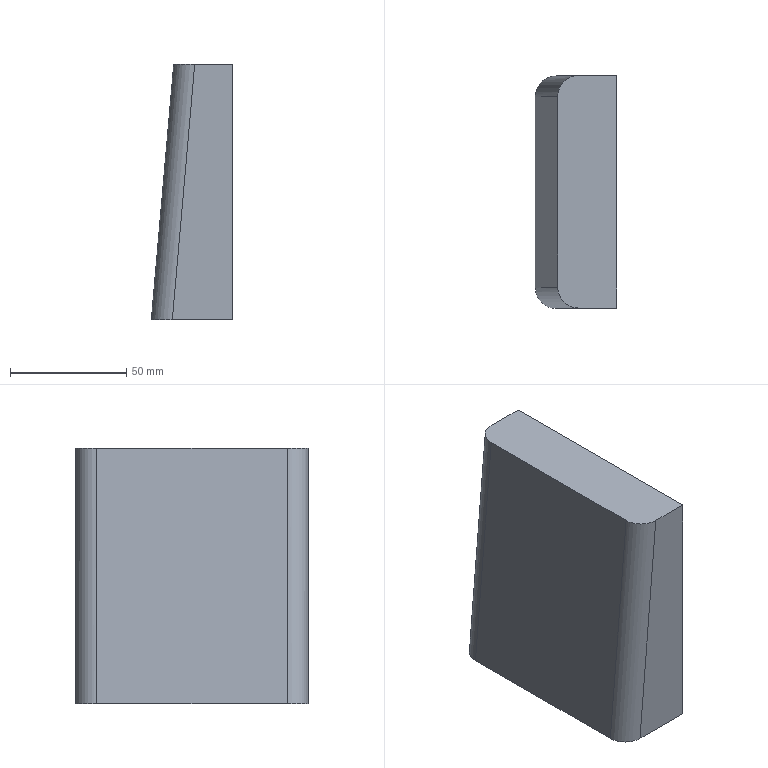Part | Creo | 1 solid | 8 faces | box 35 x 100 x 110 mm | volume 328231 mm3 | plane 6 | cylinder 2 | commonest cylinder face diameters 18 x2
STEP:
#1=CARTESIAN_POINT('',(0.,0.,0.));
#2=DIRECTION('',(0.,0.,1.));
#3=DIRECTION('',(1.,0.,0.));
#4=AXIS2_PLACEMENT_3D('',#1,#2,#3);
#5=CARTESIAN_POINT('',(-235.275,-230.589,81.559));
#6=VERTEX_POINT('',#5);
#7=CARTESIAN_POINT('',(-235.275,-148.589,81.559));
#8=VERTEX_POINT('',#7);
#9=CARTESIAN_POINT('',(-235.275,-230.589,81.559));
#10=DIRECTION('',(0.,1.,0.));
#11=VECTOR('',#10,82.);
#12=LINE('',#9,#11);
#13=EDGE_CURVE('',#6,#8,#12,.T.);
#14=ORIENTED_EDGE('',*,*,#13,.F.);
#15=CARTESIAN_POINT('',(-244.899,-230.589,-28.441));
#16=VERTEX_POINT('',#15);
#17=CARTESIAN_POINT('',(-235.275,-230.589,81.559));
#18=DIRECTION('',(-0.08716,0.,-0.9962));
#19=VECTOR('',#18,110.42);
#20=LINE('',#17,#19);
#21=EDGE_CURVE('',#6,#16,#20,.T.);
#22=ORIENTED_EDGE('',*,*,#21,.T.);
#23=CARTESIAN_POINT('',(-244.899,-148.589,-28.441));
#24=VERTEX_POINT('',#23);
#25=CARTESIAN_POINT('',(-244.899,-230.589,-28.441));
#26=DIRECTION('',(0.,1.,0.));
#27=VECTOR('',#26,82.);
#28=LINE('',#25,#27);
#29=EDGE_CURVE('',#16,#24,#28,.T.);
#30=ORIENTED_EDGE('',*,*,#29,.T.);
#31=CARTESIAN_POINT('',(-244.899,-148.589,-28.441));
#32=DIRECTION('',(0.08716,0.,0.9962));
#33=VECTOR('',#32,110.42);
#34=LINE('',#31,#33);
#35=EDGE_CURVE('',#24,#8,#34,.T.);
#36=ORIENTED_EDGE('',*,*,#35,.T.);
#37=EDGE_LOOP('',(#14,#22,#30,#36));
#38=FACE_OUTER_BOUND('',#37,.F.);
#39=CARTESIAN_POINT('',(-244.899,-119.589,-28.441));
#40=DIRECTION('',(0.9962,0.,-0.08716));
#41=DIRECTION('',(-0.08716,0.,-0.9962));
#42=AXIS2_PLACEMENT_3D('',#39,#40,#41);
#43=PLANE('',#42);
#44=ADVANCED_FACE('',(#38),#43,.F.);
#45=CARTESIAN_POINT('',(-226.241,-139.589,81.559));
#46=VERTEX_POINT('',#45);
#47=CARTESIAN_POINT('',(-209.899,-139.589,81.559));
#48=VERTEX_POINT('',#47);
#49=CARTESIAN_POINT('',(-226.241,-139.589,81.559));
#50=DIRECTION('',(1.,0.,0.));
#51=VECTOR('',#50,16.342);
#52=LINE('',#49,#51);
#53=EDGE_CURVE('',#46,#48,#52,.T.);
#54=ORIENTED_EDGE('',*,*,#53,.T.);
#55=CARTESIAN_POINT('',(-209.899,-239.589,81.559));
#56=VERTEX_POINT('',#55);
#57=CARTESIAN_POINT('',(-209.899,-139.589,81.559));
#58=DIRECTION('',(0.,-1.,0.));
#59=VECTOR('',#58,100.);
#60=LINE('',#57,#59);
#61=EDGE_CURVE('',#48,#56,#60,.T.);
#62=ORIENTED_EDGE('',*,*,#61,.T.);
#63=CARTESIAN_POINT('',(-226.241,-239.589,81.559));
#64=VERTEX_POINT('',#63);
#65=CARTESIAN_POINT('',(-209.899,-239.589,81.559));
#66=DIRECTION('',(-1.,0.,0.));
#67=VECTOR('',#66,16.342);
#68=LINE('',#65,#67);
#69=EDGE_CURVE('',#56,#64,#68,.T.);
#70=ORIENTED_EDGE('',*,*,#69,.T.);
#71=CARTESIAN_POINT('',(-226.241,-239.589,81.559));
#72=CARTESIAN_POINT('',(-226.992,-239.589,81.559));
#73=CARTESIAN_POINT('',(-228.319,-239.412,81.559));
#74=CARTESIAN_POINT('',(-230.552,-238.64,81.559));
#75=CARTESIAN_POINT('',(-232.753,-237.084,81.559));
#76=CARTESIAN_POINT('',(-234.318,-234.892,81.559));
#77=CARTESIAN_POINT('',(-235.097,-232.665,81.559));
#78=CARTESIAN_POINT('',(-235.275,-231.341,81.559));
#79=CARTESIAN_POINT('',(-235.275,-230.589,81.559));
#80=B_SPLINE_CURVE_WITH_KNOTS('',3,(#71,#72,#73,#74,#75,#76,#77,#78,#79),.UNSPECIFIED.,.F.,.F.,(4,1,1,1,1,1,4),(0.,0.125,0.25,0.5,0.75,0.875,1.),.UNSPECIFIED.);
#81=EDGE_CURVE('',#64,#6,#80,.T.);
#82=ORIENTED_EDGE('',*,*,#81,.T.);
#83=ORIENTED_EDGE('',*,*,#13,.T.);
#84=CARTESIAN_POINT('',(-235.275,-148.589,81.559));
#85=CARTESIAN_POINT('',(-235.275,-147.838,81.559));
#86=CARTESIAN_POINT('',(-235.097,-146.513,81.559));
#87=CARTESIAN_POINT('',(-234.318,-144.286,81.559));
#88=CARTESIAN_POINT('',(-232.753,-142.095,81.559));
#89=CARTESIAN_POINT('',(-230.552,-140.538,81.559));
#90=CARTESIAN_POINT('',(-228.319,-139.766,81.559));
#91=CARTESIAN_POINT('',(-226.992,-139.589,81.559));
#92=CARTESIAN_POINT('',(-226.241,-139.589,81.559));
#93=B_SPLINE_CURVE_WITH_KNOTS('',3,(#84,#85,#86,#87,#88,#89,#90,#91,#92),.UNSPECIFIED.,.F.,.F.,(4,1,1,1,1,1,4),(0.,0.125,0.25,0.5,0.75,0.875,1.),.UNSPECIFIED.);
#94=EDGE_CURVE('',#8,#46,#93,.T.);
#95=ORIENTED_EDGE('',*,*,#94,.T.);
#96=EDGE_LOOP('',(#54,#62,#70,#82,#83,#95));
#97=FACE_OUTER_BOUND('',#96,.F.);
#98=CARTESIAN_POINT('',(-244.899,-239.589,81.559));
#99=DIRECTION('',(0.,0.,-1.));
#100=DIRECTION('',(-1.,0.,0.));
#101=AXIS2_PLACEMENT_3D('',#98,#99,#100);
#102=PLANE('',#101);
#103=ADVANCED_FACE('',(#97),#102,.F.);
#104=CARTESIAN_POINT('',(-235.865,-139.589,-28.441));
#105=VERTEX_POINT('',#104);
#106=CARTESIAN_POINT('',(-209.899,-139.589,-28.441));
#107=VERTEX_POINT('',#106);
#108=CARTESIAN_POINT('',(-235.865,-139.589,-28.441));
#109=DIRECTION('',(1.,0.,0.));
#110=VECTOR('',#109,25.966);
#111=LINE('',#108,#110);
#112=EDGE_CURVE('',#105,#107,#111,.T.);
#113=ORIENTED_EDGE('',*,*,#112,.T.);
#114=CARTESIAN_POINT('',(-209.899,-139.589,-28.441));
#115=DIRECTION('',(0.,0.,1.));
#116=VECTOR('',#115,110.);
#117=LINE('',#114,#116);
#118=EDGE_CURVE('',#107,#48,#117,.T.);
#119=ORIENTED_EDGE('',*,*,#118,.T.);
#120=ORIENTED_EDGE('',*,*,#53,.F.);
#121=CARTESIAN_POINT('',(-235.865,-139.589,-28.441));
#122=DIRECTION('',(0.08716,0.,0.9962));
#123=VECTOR('',#122,110.42);
#124=LINE('',#121,#123);
#125=EDGE_CURVE('',#105,#46,#124,.T.);
#126=ORIENTED_EDGE('',*,*,#125,.F.);
#127=EDGE_LOOP('',(#113,#119,#120,#126));
#128=FACE_OUTER_BOUND('',#127,.F.);
#129=CARTESIAN_POINT('',(-209.899,-139.589,51.559));
#130=DIRECTION('',(0.,1.,0.));
#131=DIRECTION('',(0.,0.,1.));
#132=AXIS2_PLACEMENT_3D('',#129,#130,#131);
#133=PLANE('',#132);
#134=ADVANCED_FACE('',(#128),#133,.T.);
#135=ORIENTED_EDGE('',*,*,#29,.F.);
#136=CARTESIAN_POINT('',(-235.865,-239.589,-28.441));
#137=VERTEX_POINT('',#136);
#138=CARTESIAN_POINT('',(-244.899,-230.589,-28.441));
#139=CARTESIAN_POINT('',(-244.899,-231.341,-28.441));
#140=CARTESIAN_POINT('',(-244.721,-232.665,-28.441));
#141=CARTESIAN_POINT('',(-243.942,-234.892,-28.441));
#142=CARTESIAN_POINT('',(-242.376,-237.084,-28.441));
#143=CARTESIAN_POINT('',(-240.176,-238.64,-28.441));
#144=CARTESIAN_POINT('',(-237.942,-239.412,-28.441));
#145=CARTESIAN_POINT('',(-236.616,-239.589,-28.441));
#146=CARTESIAN_POINT('',(-235.865,-239.589,-28.441));
#147=B_SPLINE_CURVE_WITH_KNOTS('',3,(#138,#139,#140,#141,#142,#143,#144,#145,#146),.UNSPECIFIED.,.F.,.F.,(4,1,1,1,1,1,4),(0.,0.125,0.25,0.5,0.75,0.875,1.),.UNSPECIFIED.);
#148=EDGE_CURVE('',#16,#137,#147,.T.);
#149=ORIENTED_EDGE('',*,*,#148,.T.);
#150=CARTESIAN_POINT('',(-209.899,-239.589,-28.441));
#151=VERTEX_POINT('',#150);
#152=CARTESIAN_POINT('',(-209.899,-239.589,-28.441));
#153=DIRECTION('',(-1.,0.,0.));
#154=VECTOR('',#153,25.966);
#155=LINE('',#152,#154);
#156=EDGE_CURVE('',#151,#137,#155,.T.);
#157=ORIENTED_EDGE('',*,*,#156,.F.);
#158=CARTESIAN_POINT('',(-209.899,-139.589,-28.441));
#159=DIRECTION('',(0.,-1.,0.));
#160=VECTOR('',#159,100.);
#161=LINE('',#158,#160);
#162=EDGE_CURVE('',#107,#151,#161,.T.);
#163=ORIENTED_EDGE('',*,*,#162,.F.);
#164=ORIENTED_EDGE('',*,*,#112,.F.);
#165=CARTESIAN_POINT('',(-235.865,-139.589,-28.441));
#166=CARTESIAN_POINT('',(-236.616,-139.589,-28.441));
#167=CARTESIAN_POINT('',(-237.942,-139.766,-28.441));
#168=CARTESIAN_POINT('',(-240.176,-140.538,-28.441));
#169=CARTESIAN_POINT('',(-242.376,-142.095,-28.441));
#170=CARTESIAN_POINT('',(-243.942,-144.286,-28.441));
#171=CARTESIAN_POINT('',(-244.721,-146.513,-28.441));
#172=CARTESIAN_POINT('',(-244.899,-147.838,-28.441));
#173=CARTESIAN_POINT('',(-244.899,-148.589,-28.441));
#174=B_SPLINE_CURVE_WITH_KNOTS('',3,(#165,#166,#167,#168,#169,#170,#171,#172,#173),.UNSPECIFIED.,.F.,.F.,(4,1,1,1,1,1,4),(0.,0.125,0.25,0.5,0.75,0.875,1.),.UNSPECIFIED.);
#175=EDGE_CURVE('',#105,#24,#174,.T.);
#176=ORIENTED_EDGE('',*,*,#175,.T.);
#177=EDGE_LOOP('',(#135,#149,#157,#163,#164,#176));
#178=FACE_OUTER_BOUND('',#177,.F.);
#179=CARTESIAN_POINT('',(-244.899,-239.589,-28.441));
#180=DIRECTION('',(0.,0.,-1.));
#181=DIRECTION('',(-1.,0.,0.));
#182=AXIS2_PLACEMENT_3D('',#179,#180,#181);
#183=PLANE('',#182);
#184=ADVANCED_FACE('',(#178),#183,.T.);
#185=ORIENTED_EDGE('',*,*,#81,.F.);
#186=CARTESIAN_POINT('',(-226.241,-239.589,81.559));
#187=DIRECTION('',(-0.08716,0.,-0.9962));
#188=VECTOR('',#187,110.42);
#189=LINE('',#186,#188);
#190=EDGE_CURVE('',#64,#137,#189,.T.);
#191=ORIENTED_EDGE('',*,*,#190,.T.);
#192=ORIENTED_EDGE('',*,*,#148,.F.);
#193=ORIENTED_EDGE('',*,*,#21,.F.);
#194=EDGE_LOOP('',(#185,#191,#192,#193));
#195=FACE_OUTER_BOUND('',#194,.F.);
#196=CARTESIAN_POINT('',(-228.987,-230.589,50.166));
#197=DIRECTION('',(0.08716,0.,0.9962));
#198=DIRECTION('',(0.9962,0.,-0.08716));
#199=AXIS2_PLACEMENT_3D('',#196,#197,#198);
#200=CYLINDRICAL_SURFACE('',#199,9.);
#201=ADVANCED_FACE('',(#195),#200,.T.);
#202=ORIENTED_EDGE('',*,*,#69,.F.);
#203=CARTESIAN_POINT('',(-209.899,-239.589,-28.441));
#204=DIRECTION('',(0.,0.,1.));
#205=VECTOR('',#204,110.);
#206=LINE('',#203,#205);
#207=EDGE_CURVE('',#151,#56,#206,.T.);
#208=ORIENTED_EDGE('',*,*,#207,.F.);
#209=ORIENTED_EDGE('',*,*,#156,.T.);
#210=ORIENTED_EDGE('',*,*,#190,.F.);
#211=EDGE_LOOP('',(#202,#208,#209,#210));
#212=FACE_OUTER_BOUND('',#211,.F.);
#213=CARTESIAN_POINT('',(-244.899,-239.589,51.559));
#214=DIRECTION('',(0.,-1.,0.));
#215=DIRECTION('',(0.,0.,-1.));
#216=AXIS2_PLACEMENT_3D('',#213,#214,#215);
#217=PLANE('',#216);
#218=ADVANCED_FACE('',(#212),#217,.T.);
#219=ORIENTED_EDGE('',*,*,#162,.T.);
#220=ORIENTED_EDGE('',*,*,#207,.T.);
#221=ORIENTED_EDGE('',*,*,#61,.F.);
#222=ORIENTED_EDGE('',*,*,#118,.F.);
#223=EDGE_LOOP('',(#219,#220,#221,#222));
#224=FACE_OUTER_BOUND('',#223,.F.);
#225=CARTESIAN_POINT('',(-209.899,-239.589,51.559));
#226=DIRECTION('',(1.,0.,0.));
#227=DIRECTION('',(0.,0.,-1.));
#228=AXIS2_PLACEMENT_3D('',#225,#226,#227);
#229=PLANE('',#228);
#230=ADVANCED_FACE('',(#224),#229,.T.);
#231=ORIENTED_EDGE('',*,*,#94,.F.);
#232=ORIENTED_EDGE('',*,*,#35,.F.);
#233=ORIENTED_EDGE('',*,*,#175,.F.);
#234=ORIENTED_EDGE('',*,*,#125,.T.);
#235=EDGE_LOOP('',(#231,#232,#233,#234));
#236=FACE_OUTER_BOUND('',#235,.F.);
#237=CARTESIAN_POINT('',(-235.933,-148.589,-29.226));
#238=DIRECTION('',(0.08716,0.,0.9962));
#239=DIRECTION('',(0.9962,0.,-0.08716));
#240=AXIS2_PLACEMENT_3D('',#237,#238,#239);
#241=CYLINDRICAL_SURFACE('',#240,9.);
#242=ADVANCED_FACE('',(#236),#241,.T.);
#243=CLOSED_SHELL('',(#44,#103,#134,#184,#201,#218,#230,#242));
#244=MANIFOLD_SOLID_BREP('',#243);
#245=(LENGTH_UNIT()NAMED_UNIT(*)SI_UNIT(.MILLI.,.METRE.));
#246=UNCERTAINTY_MEASURE_WITH_UNIT(LENGTH_MEASURE(0.01539),#245,'','');
#247=(NAMED_UNIT(*)PLANE_ANGLE_UNIT()SI_UNIT($,.RADIAN.));
#248=PLANE_ANGLE_MEASURE_WITH_UNIT(PLANE_ANGLE_MEASURE(0.01745),#247);
#249=(CONVERSION_BASED_UNIT('DEGREE',#248)NAMED_UNIT(*)PLANE_ANGLE_UNIT());
#250=(NAMED_UNIT(*)SI_UNIT($,.STERADIAN.)SOLID_ANGLE_UNIT());
#251=(GEOMETRIC_REPRESENTATION_CONTEXT(3)GLOBAL_UNCERTAINTY_ASSIGNED_CONTEXT((#246))GLOBAL_UNIT_ASSIGNED_CONTEXT((#245,#249,#250))REPRESENTATION_CONTEXT('',''));
#252=ADVANCED_BREP_SHAPE_REPRESENTATION('',(#4,#244),#251);